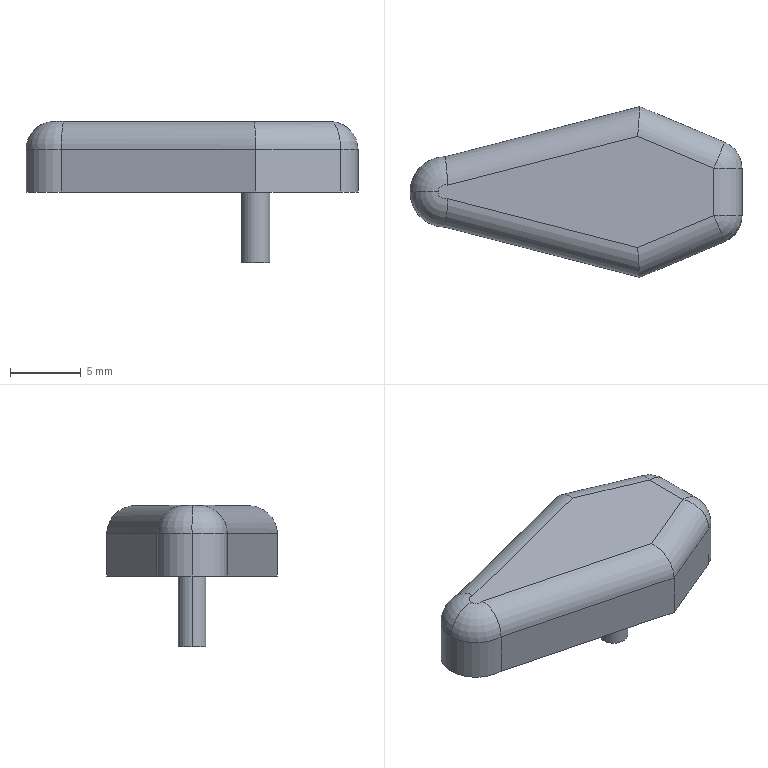Part | SolidWorks | features Fillet 3, Extrusion 1, ICE 1 | 1 solid | 23 faces | box 23.543 x 12.102 x 10 mm | volume 933.083 mm3 | cylinder 11 | plane 8 | torus 2 | sphere 2 | commonest cylinder face diameters 4 x7 2 x2 5 x2
STEP:
#1=CARTESIAN_POINT('',(-2.5,0.,3.));
#2=VERTEX_POINT('',#1);
#3=CARTESIAN_POINT('',(0.,2.5,3.));
#4=VERTEX_POINT('',#3);
#5=CARTESIAN_POINT('',(0.,0.,3.));
#6=DIRECTION('',(0.,0.,-1.));
#7=DIRECTION('',(1.,0.,0.));
#8=AXIS2_PLACEMENT_3D('',#5,#6,#7);
#9=CIRCLE('',#8,2.5);
#10=EDGE_CURVE('',#2,#4,#9,.T.);
#11=ORIENTED_EDGE('',*,*,#10,.F.);
#12=CARTESIAN_POINT('',(-0.5,0.,5.));
#13=VERTEX_POINT('',#12);
#14=CARTESIAN_POINT('',(-0.5,0.,3.));
#15=DIRECTION('',(0.,1.,0.));
#16=DIRECTION('',(-1.,0.,0.));
#17=AXIS2_PLACEMENT_3D('',#14,#15,#16);
#18=CIRCLE('',#17,2.);
#19=EDGE_CURVE('',#2,#13,#18,.T.);
#20=ORIENTED_EDGE('',*,*,#19,.T.);
#21=CARTESIAN_POINT('',(0.1561,0.475,5.));
#22=VERTEX_POINT('',#21);
#23=CARTESIAN_POINT('',(0.,0.,5.));
#24=DIRECTION('',(0.,0.,1.));
#25=DIRECTION('',(1.,0.,0.));
#26=AXIS2_PLACEMENT_3D('',#23,#24,#25);
#27=CIRCLE('',#26,0.5);
#28=EDGE_CURVE('',#22,#13,#27,.T.);
#29=ORIENTED_EDGE('',*,*,#28,.F.);
#30=CARTESIAN_POINT('',(0.,2.5,3.));
#31=CARTESIAN_POINT('',(0.,2.5,3.133));
#32=CARTESIAN_POINT('',(0.001676,2.487,3.264));
#33=CARTESIAN_POINT('',(0.008164,2.435,3.522));
#34=CARTESIAN_POINT('',(0.01306,2.396,3.65));
#35=CARTESIAN_POINT('',(0.02554,2.294,3.893));
#36=CARTESIAN_POINT('',(0.03307,2.232,4.009));
#37=CARTESIAN_POINT('',(0.05029,2.084,4.227));
#38=CARTESIAN_POINT('',(0.06004,1.999,4.33));
#39=CARTESIAN_POINT('',(0.0903,1.718,4.606));
#40=CARTESIAN_POINT('',(0.1129,1.493,4.753));
#41=CARTESIAN_POINT('',(0.1489,1.006,4.949));
#42=CARTESIAN_POINT('',(0.1643,0.7376,5.));
#43=CARTESIAN_POINT('',(0.1561,0.475,5.));
#44=B_SPLINE_CURVE_WITH_KNOTS('',3,(#30,#31,#32,#33,#34,#35,#36,#37,#38,#39,#40,#41,#42,#43),.UNSPECIFIED.,.F.,.F.,(4,2,2,2,2,2,4),(0.,0.0003941,0.0007882,0.001182,0.001576,0.002364,0.003153),.UNSPECIFIED.);
#45=EDGE_CURVE('',#4,#22,#44,.T.);
#46=ORIENTED_EDGE('',*,*,#45,.F.);
#47=EDGE_LOOP('',(#11,#20,#29,#46));
#48=FACE_OUTER_BOUND('',#47,.T.);
#49=CARTESIAN_POINT('',(0.,0.,3.));
#50=DIRECTION('',(0.,0.,1.));
#51=DIRECTION('',(1.,0.,0.));
#52=AXIS2_PLACEMENT_3D('',#49,#50,#51);
#53=TOROIDAL_SURFACE('',#52,0.5,2.);
#54=ADVANCED_FACE('',(#48),#53,.T.);
#55=CARTESIAN_POINT('',(12.798,0.,-5.));
#56=VERTEX_POINT('',#55);
#57=CARTESIAN_POINT('',(14.798,0.,-5.));
#58=VERTEX_POINT('',#57);
#59=CARTESIAN_POINT('',(13.798,0.,-5.));
#60=DIRECTION('',(0.,0.,-1.));
#61=DIRECTION('',(-1.,0.,0.));
#62=AXIS2_PLACEMENT_3D('',#59,#60,#61);
#63=CIRCLE('',#62,1.);
#64=EDGE_CURVE('',#56,#58,#63,.T.);
#65=ORIENTED_EDGE('',*,*,#64,.F.);
#66=CARTESIAN_POINT('',(12.798,0.,0.));
#67=VERTEX_POINT('',#66);
#68=CARTESIAN_POINT('',(12.798,0.,-5.));
#69=DIRECTION('',(0.,0.,1.));
#70=VECTOR('',#69,1000.);
#71=LINE('',#68,#70);
#72=EDGE_CURVE('',#56,#67,#71,.T.);
#73=ORIENTED_EDGE('',*,*,#72,.T.);
#74=CARTESIAN_POINT('',(14.798,0.,0.));
#75=VERTEX_POINT('',#74);
#76=CARTESIAN_POINT('',(13.798,0.,0.));
#77=DIRECTION('',(0.,0.,-1.));
#78=DIRECTION('',(1.,0.,0.));
#79=AXIS2_PLACEMENT_3D('',#76,#77,#78);
#80=CIRCLE('',#79,1.);
#81=EDGE_CURVE('',#67,#75,#80,.T.);
#82=ORIENTED_EDGE('',*,*,#81,.T.);
#83=CARTESIAN_POINT('',(14.798,0.,-5.));
#84=DIRECTION('',(0.,0.,1.));
#85=VECTOR('',#84,1000.);
#86=LINE('',#83,#85);
#87=EDGE_CURVE('',#58,#75,#86,.T.);
#88=ORIENTED_EDGE('',*,*,#87,.F.);
#89=EDGE_LOOP('',(#65,#73,#82,#88));
#90=FACE_OUTER_BOUND('',#89,.T.);
#91=CARTESIAN_POINT('',(13.798,0.,-5.));
#92=DIRECTION('',(0.,0.,1.));
#93=DIRECTION('',(1.,0.,0.));
#94=AXIS2_PLACEMENT_3D('',#91,#92,#93);
#95=CYLINDRICAL_SURFACE('',#94,1.);
#96=ADVANCED_FACE('',(#90),#95,.T.);
#97=CARTESIAN_POINT('',(0.,-2.5,3.));
#98=VERTEX_POINT('',#97);
#99=CARTESIAN_POINT('',(0.,0.,3.));
#100=DIRECTION('',(0.,0.,-1.));
#101=DIRECTION('',(1.,0.,0.));
#102=AXIS2_PLACEMENT_3D('',#99,#100,#101);
#103=CIRCLE('',#102,2.5);
#104=EDGE_CURVE('',#98,#2,#103,.T.);
#105=ORIENTED_EDGE('',*,*,#104,.T.);
#106=CARTESIAN_POINT('',(-2.5,0.,0.));
#107=VERTEX_POINT('',#106);
#108=CARTESIAN_POINT('',(-2.5,0.,5.));
#109=DIRECTION('',(0.,0.,-1.));
#110=VECTOR('',#109,1000.);
#111=LINE('',#108,#110);
#112=EDGE_CURVE('',#2,#107,#111,.T.);
#113=ORIENTED_EDGE('',*,*,#112,.T.);
#114=CARTESIAN_POINT('',(0.,-2.5,0.));
#115=VERTEX_POINT('',#114);
#116=CARTESIAN_POINT('',(0.,0.,0.));
#117=DIRECTION('',(0.,0.,1.));
#118=DIRECTION('',(1.,0.,0.));
#119=AXIS2_PLACEMENT_3D('',#116,#117,#118);
#120=CIRCLE('',#119,2.5);
#121=EDGE_CURVE('',#107,#115,#120,.T.);
#122=ORIENTED_EDGE('',*,*,#121,.T.);
#123=CARTESIAN_POINT('',(0.,-2.5,5.));
#124=DIRECTION('',(0.,0.,-1.));
#125=VECTOR('',#124,1000.);
#126=LINE('',#123,#125);
#127=EDGE_CURVE('',#98,#115,#126,.T.);
#128=ORIENTED_EDGE('',*,*,#127,.F.);
#129=EDGE_LOOP('',(#105,#113,#122,#128));
#130=FACE_OUTER_BOUND('',#129,.T.);
#131=CARTESIAN_POINT('',(0.,0.,5.));
#132=DIRECTION('',(0.,0.,-1.));
#133=DIRECTION('',(-1.,0.,0.));
#134=AXIS2_PLACEMENT_3D('',#131,#132,#133);
#135=CYLINDRICAL_SURFACE('',#134,2.5);
#136=ADVANCED_FACE('',(#130),#135,.T.);
#137=ORIENTED_EDGE('',*,*,#112,.F.);
#138=ORIENTED_EDGE('',*,*,#10,.T.);
#139=CARTESIAN_POINT('',(0.,2.5,0.));
#140=VERTEX_POINT('',#139);
#141=CARTESIAN_POINT('',(0.,2.5,5.));
#142=DIRECTION('',(0.,0.,-1.));
#143=VECTOR('',#142,1000.);
#144=LINE('',#141,#143);
#145=EDGE_CURVE('',#4,#140,#144,.T.);
#146=ORIENTED_EDGE('',*,*,#145,.T.);
#147=CARTESIAN_POINT('',(0.,0.,0.));
#148=DIRECTION('',(0.,0.,1.));
#149=DIRECTION('',(1.,0.,0.));
#150=AXIS2_PLACEMENT_3D('',#147,#148,#149);
#151=CIRCLE('',#150,2.5);
#152=EDGE_CURVE('',#140,#107,#151,.T.);
#153=ORIENTED_EDGE('',*,*,#152,.T.);
#154=EDGE_LOOP('',(#137,#138,#146,#153));
#155=FACE_OUTER_BOUND('',#154,.T.);
#156=CARTESIAN_POINT('',(0.,0.,5.));
#157=DIRECTION('',(0.,0.,-1.));
#158=DIRECTION('',(-1.,0.,0.));
#159=AXIS2_PLACEMENT_3D('',#156,#157,#158);
#160=CYLINDRICAL_SURFACE('',#159,2.5);
#161=ADVANCED_FACE('',(#155),#160,.T.);
#162=CARTESIAN_POINT('',(13.798,-6.051,3.));
#163=VERTEX_POINT('',#162);
#164=CARTESIAN_POINT('',(13.798,-6.051,0.));
#165=VERTEX_POINT('',#164);
#166=CARTESIAN_POINT('',(13.798,-6.051,5.));
#167=DIRECTION('',(0.,0.,-1.));
#168=VECTOR('',#167,1000.);
#169=LINE('',#166,#168);
#170=EDGE_CURVE('',#163,#165,#169,.T.);
#171=ORIENTED_EDGE('',*,*,#170,.F.);
#172=CARTESIAN_POINT('',(0.,-2.5,3.));
#173=DIRECTION('',(-0.9684,0.2492,0.));
#174=VECTOR('',#173,1000.);
#175=LINE('',#172,#174);
#176=EDGE_CURVE('',#163,#98,#175,.T.);
#177=ORIENTED_EDGE('',*,*,#176,.T.);
#178=ORIENTED_EDGE('',*,*,#127,.T.);
#179=CARTESIAN_POINT('',(0.,-2.5,0.));
#180=DIRECTION('',(0.9684,-0.2492,0.));
#181=VECTOR('',#180,1000.);
#182=LINE('',#179,#181);
#183=EDGE_CURVE('',#115,#165,#182,.T.);
#184=ORIENTED_EDGE('',*,*,#183,.T.);
#185=EDGE_LOOP('',(#171,#177,#178,#184));
#186=FACE_OUTER_BOUND('',#185,.T.);
#187=CARTESIAN_POINT('',(0.,-2.5,5.));
#188=DIRECTION('',(0.2492,0.9684,0.));
#189=DIRECTION('',(-0.9684,0.2492,0.));
#190=AXIS2_PLACEMENT_3D('',#187,#188,#189);
#191=PLANE('',#190);
#192=ADVANCED_FACE('',(#186),#191,.F.);
#193=CARTESIAN_POINT('',(19.816,-3.528,0.));
#194=VERTEX_POINT('',#193);
#195=CARTESIAN_POINT('',(13.798,-6.051,0.));
#196=DIRECTION('',(0.9223,0.3866,0.));
#197=VECTOR('',#196,1000.);
#198=LINE('',#195,#197);
#199=EDGE_CURVE('',#165,#194,#198,.T.);
#200=ORIENTED_EDGE('',*,*,#199,.T.);
#201=CARTESIAN_POINT('',(19.816,-3.528,3.));
#202=VERTEX_POINT('',#201);
#203=CARTESIAN_POINT('',(19.816,-3.528,5.));
#204=DIRECTION('',(0.,0.,1.));
#205=VECTOR('',#204,1000.);
#206=LINE('',#203,#205);
#207=EDGE_CURVE('',#194,#202,#206,.T.);
#208=ORIENTED_EDGE('',*,*,#207,.T.);
#209=CARTESIAN_POINT('',(13.798,-6.051,3.));
#210=DIRECTION('',(-0.9223,-0.3866,0.));
#211=VECTOR('',#210,1000.);
#212=LINE('',#209,#211);
#213=EDGE_CURVE('',#202,#163,#212,.T.);
#214=ORIENTED_EDGE('',*,*,#213,.T.);
#215=ORIENTED_EDGE('',*,*,#170,.T.);
#216=EDGE_LOOP('',(#200,#208,#214,#215));
#217=FACE_OUTER_BOUND('',#216,.T.);
#218=CARTESIAN_POINT('',(13.798,-6.051,5.));
#219=DIRECTION('',(-0.3866,0.9223,0.));
#220=DIRECTION('',(-0.9223,-0.3866,0.));
#221=AXIS2_PLACEMENT_3D('',#218,#219,#220);
#222=PLANE('',#221);
#223=ADVANCED_FACE('',(#217),#222,.F.);
#224=CARTESIAN_POINT('',(21.043,-1.684,0.));
#225=VERTEX_POINT('',#224);
#226=CARTESIAN_POINT('',(21.043,1.684,0.));
#227=VERTEX_POINT('',#226);
#228=CARTESIAN_POINT('',(21.043,3.014,0.));
#229=DIRECTION('',(0.,1.,0.));
#230=VECTOR('',#229,1000.);
#231=LINE('',#228,#230);
#232=EDGE_CURVE('',#225,#227,#231,.T.);
#233=ORIENTED_EDGE('',*,*,#232,.T.);
#234=CARTESIAN_POINT('',(21.043,1.684,3.));
#235=VERTEX_POINT('',#234);
#236=CARTESIAN_POINT('',(21.043,1.684,5.));
#237=DIRECTION('',(0.,0.,1.));
#238=VECTOR('',#237,1000.);
#239=LINE('',#236,#238);
#240=EDGE_CURVE('',#227,#235,#239,.T.);
#241=ORIENTED_EDGE('',*,*,#240,.T.);
#242=CARTESIAN_POINT('',(21.043,-1.684,3.));
#243=VERTEX_POINT('',#242);
#244=CARTESIAN_POINT('',(21.043,-3.014,3.));
#245=DIRECTION('',(0.,-1.,0.));
#246=VECTOR('',#245,1000.);
#247=LINE('',#244,#246);
#248=EDGE_CURVE('',#235,#243,#247,.T.);
#249=ORIENTED_EDGE('',*,*,#248,.T.);
#250=CARTESIAN_POINT('',(21.043,-1.684,5.));
#251=DIRECTION('',(0.,0.,-1.));
#252=VECTOR('',#251,1000.);
#253=LINE('',#250,#252);
#254=EDGE_CURVE('',#243,#225,#253,.T.);
#255=ORIENTED_EDGE('',*,*,#254,.T.);
#256=EDGE_LOOP('',(#233,#241,#249,#255));
#257=FACE_OUTER_BOUND('',#256,.T.);
#258=CARTESIAN_POINT('',(21.043,3.014,5.));
#259=DIRECTION('',(-1.,0.,0.));
#260=DIRECTION('',(0.,0.,1.));
#261=AXIS2_PLACEMENT_3D('',#258,#259,#260);
#262=PLANE('',#261);
#263=ADVANCED_FACE('',(#257),#262,.F.);
#264=CARTESIAN_POINT('',(13.798,6.051,3.));
#265=VERTEX_POINT('',#264);
#266=CARTESIAN_POINT('',(19.816,3.528,3.));
#267=VERTEX_POINT('',#266);
#268=CARTESIAN_POINT('',(19.043,3.852,3.));
#269=DIRECTION('',(0.9223,-0.3866,0.));
#270=VECTOR('',#269,1000.);
#271=LINE('',#268,#270);
#272=EDGE_CURVE('',#265,#267,#271,.T.);
#273=ORIENTED_EDGE('',*,*,#272,.T.);
#274=CARTESIAN_POINT('',(19.816,3.528,0.));
#275=VERTEX_POINT('',#274);
#276=CARTESIAN_POINT('',(19.816,3.528,5.));
#277=DIRECTION('',(0.,0.,-1.));
#278=VECTOR('',#277,1000.);
#279=LINE('',#276,#278);
#280=EDGE_CURVE('',#267,#275,#279,.T.);
#281=ORIENTED_EDGE('',*,*,#280,.T.);
#282=CARTESIAN_POINT('',(13.798,6.051,0.));
#283=VERTEX_POINT('',#282);
#284=CARTESIAN_POINT('',(13.798,6.051,0.));
#285=DIRECTION('',(-0.9223,0.3866,0.));
#286=VECTOR('',#285,1000.);
#287=LINE('',#284,#286);
#288=EDGE_CURVE('',#275,#283,#287,.T.);
#289=ORIENTED_EDGE('',*,*,#288,.T.);
#290=CARTESIAN_POINT('',(13.798,6.051,5.));
#291=DIRECTION('',(0.,0.,-1.));
#292=VECTOR('',#291,1000.);
#293=LINE('',#290,#292);
#294=EDGE_CURVE('',#265,#283,#293,.T.);
#295=ORIENTED_EDGE('',*,*,#294,.F.);
#296=EDGE_LOOP('',(#273,#281,#289,#295));
#297=FACE_OUTER_BOUND('',#296,.T.);
#298=CARTESIAN_POINT('',(13.798,6.051,5.));
#299=DIRECTION('',(-0.3866,-0.9223,0.));
#300=DIRECTION('',(0.9223,-0.3866,0.));
#301=AXIS2_PLACEMENT_3D('',#298,#299,#300);
#302=PLANE('',#301);
#303=ADVANCED_FACE('',(#297),#302,.F.);
#304=ORIENTED_EDGE('',*,*,#145,.F.);
#305=CARTESIAN_POINT('',(13.798,6.051,3.));
#306=DIRECTION('',(0.9684,0.2492,0.));
#307=VECTOR('',#306,1000.);
#308=LINE('',#305,#307);
#309=EDGE_CURVE('',#4,#265,#308,.T.);
#310=ORIENTED_EDGE('',*,*,#309,.T.);
#311=ORIENTED_EDGE('',*,*,#294,.T.);
#312=CARTESIAN_POINT('',(0.,2.5,0.));
#313=DIRECTION('',(-0.9684,-0.2492,0.));
#314=VECTOR('',#313,1000.);
#315=LINE('',#312,#314);
#316=EDGE_CURVE('',#283,#140,#315,.T.);
#317=ORIENTED_EDGE('',*,*,#316,.T.);
#318=EDGE_LOOP('',(#304,#310,#311,#317));
#319=FACE_OUTER_BOUND('',#318,.T.);
#320=CARTESIAN_POINT('',(0.,2.5,5.));
#321=DIRECTION('',(0.2492,-0.9684,0.));
#322=DIRECTION('',(0.9684,0.2492,0.));
#323=AXIS2_PLACEMENT_3D('',#320,#321,#322);
#324=PLANE('',#323);
#325=ADVANCED_FACE('',(#319),#324,.F.);
#326=ORIENTED_EDGE('',*,*,#28,.T.);
#327=CARTESIAN_POINT('',(0.1561,-0.475,5.));
#328=VERTEX_POINT('',#327);
#329=CARTESIAN_POINT('',(0.,0.,5.));
#330=DIRECTION('',(0.,0.,1.));
#331=DIRECTION('',(1.,0.,0.));
#332=AXIS2_PLACEMENT_3D('',#329,#330,#331);
#333=CIRCLE('',#332,0.5);
#334=EDGE_CURVE('',#13,#328,#333,.T.);
#335=ORIENTED_EDGE('',*,*,#334,.T.);
#336=CARTESIAN_POINT('',(13.645,-3.946,5.));
#337=VERTEX_POINT('',#336);
#338=CARTESIAN_POINT('',(14.296,-4.114,5.));
#339=DIRECTION('',(0.9684,-0.2492,0.));
#340=VECTOR('',#339,1000.);
#341=LINE('',#338,#340);
#342=EDGE_CURVE('',#328,#337,#341,.T.);
#343=ORIENTED_EDGE('',*,*,#342,.T.);
#344=CARTESIAN_POINT('',(19.043,-1.684,5.));
#345=VERTEX_POINT('',#344);
#346=CARTESIAN_POINT('',(18.27,-2.008,5.));
#347=DIRECTION('',(0.9223,0.3866,0.));
#348=VECTOR('',#347,1000.);
#349=LINE('',#346,#348);
#350=EDGE_CURVE('',#337,#345,#349,.T.);
#351=ORIENTED_EDGE('',*,*,#350,.T.);
#352=CARTESIAN_POINT('',(19.043,1.684,5.));
#353=VERTEX_POINT('',#352);
#354=CARTESIAN_POINT('',(19.043,3.014,5.));
#355=DIRECTION('',(0.,1.,0.));
#356=VECTOR('',#355,1000.);
#357=LINE('',#354,#356);
#358=EDGE_CURVE('',#345,#353,#357,.T.);
#359=ORIENTED_EDGE('',*,*,#358,.T.);
#360=CARTESIAN_POINT('',(13.645,3.946,5.));
#361=VERTEX_POINT('',#360);
#362=CARTESIAN_POINT('',(13.025,4.206,5.));
#363=DIRECTION('',(-0.9223,0.3866,0.));
#364=VECTOR('',#363,1000.);
#365=LINE('',#362,#364);
#366=EDGE_CURVE('',#353,#361,#365,.T.);
#367=ORIENTED_EDGE('',*,*,#366,.T.);
#368=CARTESIAN_POINT('',(0.4985,0.5631,5.));
#369=DIRECTION('',(-0.9684,-0.2492,0.));
#370=VECTOR('',#369,1000.);
#371=LINE('',#368,#370);
#372=EDGE_CURVE('',#361,#22,#371,.T.);
#373=ORIENTED_EDGE('',*,*,#372,.T.);
#374=EDGE_LOOP('',(#326,#335,#343,#351,#359,#367,#373));
#375=FACE_OUTER_BOUND('',#374,.T.);
#376=CARTESIAN_POINT('',(0.,0.,5.));
#377=DIRECTION('',(0.,0.,1.));
#378=DIRECTION('',(1.,0.,0.));
#379=AXIS2_PLACEMENT_3D('',#376,#377,#378);
#380=PLANE('',#379);
#381=ADVANCED_FACE('',(#375),#380,.T.);
#382=CARTESIAN_POINT('',(13.798,0.,0.));
#383=DIRECTION('',(0.,0.,-1.));
#384=DIRECTION('',(1.,0.,0.));
#385=AXIS2_PLACEMENT_3D('',#382,#383,#384);
#386=CIRCLE('',#385,1.);
#387=EDGE_CURVE('',#75,#67,#386,.T.);
#388=ORIENTED_EDGE('',*,*,#387,.F.);
#389=ORIENTED_EDGE('',*,*,#81,.F.);
#390=EDGE_LOOP('',(#388,#389));
#391=FACE_BOUND('',#390,.T.);
#392=ORIENTED_EDGE('',*,*,#288,.F.);
#393=CARTESIAN_POINT('',(19.043,1.684,0.));
#394=DIRECTION('',(0.,0.,-1.));
#395=DIRECTION('',(1.,0.,0.));
#396=AXIS2_PLACEMENT_3D('',#393,#394,#395);
#397=CIRCLE('',#396,2.);
#398=EDGE_CURVE('',#275,#227,#397,.T.);
#399=ORIENTED_EDGE('',*,*,#398,.T.);
#400=ORIENTED_EDGE('',*,*,#232,.F.);
#401=CARTESIAN_POINT('',(19.043,-1.684,0.));
#402=DIRECTION('',(0.,0.,-1.));
#403=DIRECTION('',(1.,0.,0.));
#404=AXIS2_PLACEMENT_3D('',#401,#402,#403);
#405=CIRCLE('',#404,2.);
#406=EDGE_CURVE('',#225,#194,#405,.T.);
#407=ORIENTED_EDGE('',*,*,#406,.T.);
#408=ORIENTED_EDGE('',*,*,#199,.F.);
#409=ORIENTED_EDGE('',*,*,#183,.F.);
#410=ORIENTED_EDGE('',*,*,#121,.F.);
#411=ORIENTED_EDGE('',*,*,#152,.F.);
#412=ORIENTED_EDGE('',*,*,#316,.F.);
#413=EDGE_LOOP('',(#392,#399,#400,#407,#408,#409,#410,#411,#412));
#414=FACE_OUTER_BOUND('',#413,.T.);
#415=CARTESIAN_POINT('',(0.,0.,0.));
#416=DIRECTION('',(0.,0.,1.));
#417=DIRECTION('',(1.,0.,0.));
#418=AXIS2_PLACEMENT_3D('',#415,#416,#417);
#419=PLANE('',#418);
#420=ADVANCED_FACE('',(#391,#414),#419,.F.);
#421=ORIENTED_EDGE('',*,*,#72,.F.);
#422=CARTESIAN_POINT('',(13.798,0.,-5.));
#423=DIRECTION('',(0.,0.,-1.));
#424=DIRECTION('',(-1.,0.,0.));
#425=AXIS2_PLACEMENT_3D('',#422,#423,#424);
#426=CIRCLE('',#425,1.);
#427=EDGE_CURVE('',#58,#56,#426,.T.);
#428=ORIENTED_EDGE('',*,*,#427,.F.);
#429=ORIENTED_EDGE('',*,*,#87,.T.);
#430=ORIENTED_EDGE('',*,*,#387,.T.);
#431=EDGE_LOOP('',(#421,#428,#429,#430));
#432=FACE_OUTER_BOUND('',#431,.T.);
#433=CARTESIAN_POINT('',(13.798,0.,-5.));
#434=DIRECTION('',(0.,0.,1.));
#435=DIRECTION('',(1.,0.,0.));
#436=AXIS2_PLACEMENT_3D('',#433,#434,#435);
#437=CYLINDRICAL_SURFACE('',#436,1.);
#438=ADVANCED_FACE('',(#432),#437,.T.);
#439=ORIENTED_EDGE('',*,*,#427,.T.);
#440=ORIENTED_EDGE('',*,*,#64,.T.);
#441=EDGE_LOOP('',(#439,#440));
#442=FACE_OUTER_BOUND('',#441,.T.);
#443=CARTESIAN_POINT('',(13.798,0.,-5.));
#444=DIRECTION('',(0.,0.,-1.));
#445=DIRECTION('',(-1.,0.,0.));
#446=AXIS2_PLACEMENT_3D('',#443,#444,#445);
#447=PLANE('',#446);
#448=ADVANCED_FACE('',(#442),#447,.T.);
#449=ORIENTED_EDGE('',*,*,#248,.F.);
#450=CARTESIAN_POINT('',(19.043,1.684,3.));
#451=DIRECTION('',(0.,-1.,0.));
#452=DIRECTION('',(0.,0.,-1.));
#453=AXIS2_PLACEMENT_3D('',#450,#451,#452);
#454=CIRCLE('',#453,2.);
#455=EDGE_CURVE('',#235,#353,#454,.T.);
#456=ORIENTED_EDGE('',*,*,#455,.T.);
#457=ORIENTED_EDGE('',*,*,#358,.F.);
#458=CARTESIAN_POINT('',(19.043,-1.684,3.));
#459=DIRECTION('',(0.,1.,0.));
#460=DIRECTION('',(0.,0.,-1.));
#461=AXIS2_PLACEMENT_3D('',#458,#459,#460);
#462=CIRCLE('',#461,2.);
#463=EDGE_CURVE('',#345,#243,#462,.T.);
#464=ORIENTED_EDGE('',*,*,#463,.T.);
#465=EDGE_LOOP('',(#449,#456,#457,#464));
#466=FACE_OUTER_BOUND('',#465,.T.);
#467=CARTESIAN_POINT('',(19.043,0.,3.));
#468=DIRECTION('',(0.,-1.,0.));
#469=DIRECTION('',(0.,0.,-1.));
#470=AXIS2_PLACEMENT_3D('',#467,#468,#469);
#471=CYLINDRICAL_SURFACE('',#470,2.);
#472=ADVANCED_FACE('',(#466),#471,.T.);
#473=ORIENTED_EDGE('',*,*,#342,.F.);
#474=CARTESIAN_POINT('',(0.1561,-0.475,5.));
#475=CARTESIAN_POINT('',(0.1643,-0.7395,5.));
#476=CARTESIAN_POINT('',(0.1489,-1.006,4.949));
#477=CARTESIAN_POINT('',(0.1129,-1.493,4.753));
#478=CARTESIAN_POINT('',(0.09029,-1.718,4.606));
#479=CARTESIAN_POINT('',(0.06003,-1.999,4.33));
#480=CARTESIAN_POINT('',(0.05029,-2.084,4.227));
#481=CARTESIAN_POINT('',(0.03307,-2.232,4.009));
#482=CARTESIAN_POINT('',(0.02554,-2.294,3.893));
#483=CARTESIAN_POINT('',(0.01306,-2.396,3.65));
#484=CARTESIAN_POINT('',(0.008163,-2.435,3.522));
#485=CARTESIAN_POINT('',(0.001676,-2.487,3.264));
#486=CARTESIAN_POINT('',(0.,-2.5,3.133));
#487=CARTESIAN_POINT('',(0.,-2.5,3.));
#488=B_SPLINE_CURVE_WITH_KNOTS('',3,(#474,#475,#476,#477,#478,#479,#480,#481,#482,#483,#484,#485,#486,#487),.UNSPECIFIED.,.F.,.F.,(4,2,2,2,2,2,4),(-0.00001218,0.0007817,0.001576,0.001973,0.002369,0.002766,0.003163),.UNSPECIFIED.);
#489=EDGE_CURVE('',#328,#98,#488,.T.);
#490=ORIENTED_EDGE('',*,*,#489,.T.);
#491=ORIENTED_EDGE('',*,*,#176,.F.);
#492=CARTESIAN_POINT('',(13.645,-3.946,5.));
#493=CARTESIAN_POINT('',(13.734,-5.179,5.));
#494=CARTESIAN_POINT('',(13.798,-6.051,4.172));
#495=CARTESIAN_POINT('',(13.798,-6.051,3.));
#496=(BOUNDED_CURVE()B_SPLINE_CURVE(3,(#492,#493,#494,#495),.UNSPECIFIED.,.F.,.T.)B_SPLINE_CURVE_WITH_KNOTS((4,4),(1.571,3.142),.UNSPECIFIED.)CURVE()GEOMETRIC_REPRESENTATION_ITEM()RATIONAL_B_SPLINE_CURVE((1.,0.8047,0.8047,1.))REPRESENTATION_ITEM(''));
#497=EDGE_CURVE('',#337,#163,#496,.T.);
#498=ORIENTED_EDGE('',*,*,#497,.F.);
#499=EDGE_LOOP('',(#473,#490,#491,#498));
#500=FACE_OUTER_BOUND('',#499,.T.);
#501=CARTESIAN_POINT('',(-0.105,-0.4078,3.));
#502=DIRECTION('',(-0.9684,0.2492,0.));
#503=DIRECTION('',(-0.2492,-0.9684,0.));
#504=AXIS2_PLACEMENT_3D('',#501,#502,#503);
#505=CYLINDRICAL_SURFACE('',#504,2.);
#506=ADVANCED_FACE('',(#500),#505,.T.);
#507=CARTESIAN_POINT('',(19.043,-1.684,3.));
#508=DIRECTION('',(0.9223,0.3866,0.));
#509=DIRECTION('',(-0.3866,0.9223,0.));
#510=AXIS2_PLACEMENT_3D('',#507,#508,#509);
#511=CIRCLE('',#510,2.);
#512=EDGE_CURVE('',#345,#202,#511,.T.);
#513=ORIENTED_EDGE('',*,*,#512,.F.);
#514=ORIENTED_EDGE('',*,*,#350,.F.);
#515=ORIENTED_EDGE('',*,*,#497,.T.);
#516=ORIENTED_EDGE('',*,*,#213,.F.);
#517=EDGE_LOOP('',(#513,#514,#515,#516));
#518=FACE_OUTER_BOUND('',#517,.T.);
#519=CARTESIAN_POINT('',(3.446,-8.221,3.));
#520=DIRECTION('',(-0.9223,-0.3866,0.));
#521=DIRECTION('',(0.3866,-0.9223,0.));
#522=AXIS2_PLACEMENT_3D('',#519,#520,#521);
#523=CYLINDRICAL_SURFACE('',#522,2.);
#524=ADVANCED_FACE('',(#518),#523,.T.);
#525=ORIENTED_EDGE('',*,*,#463,.F.);
#526=ORIENTED_EDGE('',*,*,#512,.T.);
#527=CARTESIAN_POINT('',(19.043,-1.684,3.));
#528=DIRECTION('',(0.,0.,-1.));
#529=DIRECTION('',(-1.,0.,0.));
#530=AXIS2_PLACEMENT_3D('',#527,#528,#529);
#531=CIRCLE('',#530,2.);
#532=EDGE_CURVE('',#243,#202,#531,.T.);
#533=ORIENTED_EDGE('',*,*,#532,.F.);
#534=EDGE_LOOP('',(#525,#526,#533));
#535=FACE_OUTER_BOUND('',#534,.T.);
#536=CARTESIAN_POINT('',(19.043,-1.684,3.));
#537=DIRECTION('',(0.,0.,1.));
#538=DIRECTION('',(-0.9223,-0.3866,0.));
#539=AXIS2_PLACEMENT_3D('',#536,#537,#538);
#540=SPHERICAL_SURFACE('',#539,2.);
#541=ADVANCED_FACE('',(#535),#540,.T.);
#542=ORIENTED_EDGE('',*,*,#532,.T.);
#543=ORIENTED_EDGE('',*,*,#207,.F.);
#544=ORIENTED_EDGE('',*,*,#406,.F.);
#545=ORIENTED_EDGE('',*,*,#254,.F.);
#546=EDGE_LOOP('',(#542,#543,#544,#545));
#547=FACE_OUTER_BOUND('',#546,.T.);
#548=CARTESIAN_POINT('',(19.043,-1.684,5.));
#549=DIRECTION('',(0.,0.,-1.));
#550=DIRECTION('',(-1.,0.,0.));
#551=AXIS2_PLACEMENT_3D('',#548,#549,#550);
#552=CYLINDRICAL_SURFACE('',#551,2.);
#553=ADVANCED_FACE('',(#547),#552,.T.);
#554=ORIENTED_EDGE('',*,*,#19,.F.);
#555=ORIENTED_EDGE('',*,*,#104,.F.);
#556=ORIENTED_EDGE('',*,*,#489,.F.);
#557=ORIENTED_EDGE('',*,*,#334,.F.);
#558=EDGE_LOOP('',(#554,#555,#556,#557));
#559=FACE_OUTER_BOUND('',#558,.T.);
#560=CARTESIAN_POINT('',(0.,0.,3.));
#561=DIRECTION('',(0.,0.,1.));
#562=DIRECTION('',(1.,0.,0.));
#563=AXIS2_PLACEMENT_3D('',#560,#561,#562);
#564=TOROIDAL_SURFACE('',#563,0.5,2.);
#565=ADVANCED_FACE('',(#559),#564,.T.);
#566=ORIENTED_EDGE('',*,*,#45,.T.);
#567=ORIENTED_EDGE('',*,*,#372,.F.);
#568=CARTESIAN_POINT('',(13.798,6.051,3.));
#569=CARTESIAN_POINT('',(13.798,6.051,4.172));
#570=CARTESIAN_POINT('',(13.734,5.179,5.));
#571=CARTESIAN_POINT('',(13.645,3.946,5.));
#572=(BOUNDED_CURVE()B_SPLINE_CURVE(3,(#568,#569,#570,#571),.UNSPECIFIED.,.F.,.T.)B_SPLINE_CURVE_WITH_KNOTS((4,4),(3.142,4.712),.UNSPECIFIED.)CURVE()GEOMETRIC_REPRESENTATION_ITEM()RATIONAL_B_SPLINE_CURVE((1.,0.8047,0.8047,1.))REPRESENTATION_ITEM(''));
#573=EDGE_CURVE('',#265,#361,#572,.T.);
#574=ORIENTED_EDGE('',*,*,#573,.F.);
#575=ORIENTED_EDGE('',*,*,#309,.F.);
#576=EDGE_LOOP('',(#566,#567,#574,#575));
#577=FACE_OUTER_BOUND('',#576,.T.);
#578=CARTESIAN_POINT('',(-0.105,0.4078,3.));
#579=DIRECTION('',(0.9684,0.2492,0.));
#580=DIRECTION('',(-0.2492,0.9684,0.));
#581=AXIS2_PLACEMENT_3D('',#578,#579,#580);
#582=CYLINDRICAL_SURFACE('',#581,2.);
#583=ADVANCED_FACE('',(#577),#582,.T.);
#584=ORIENTED_EDGE('',*,*,#573,.T.);
#585=ORIENTED_EDGE('',*,*,#366,.F.);
#586=CARTESIAN_POINT('',(19.043,1.684,3.));
#587=DIRECTION('',(0.9223,-0.3866,0.));
#588=DIRECTION('',(0.3866,0.9223,0.));
#589=AXIS2_PLACEMENT_3D('',#586,#587,#588);
#590=CIRCLE('',#589,2.);
#591=EDGE_CURVE('',#267,#353,#590,.T.);
#592=ORIENTED_EDGE('',*,*,#591,.F.);
#593=ORIENTED_EDGE('',*,*,#272,.F.);
#594=EDGE_LOOP('',(#584,#585,#592,#593));
#595=FACE_OUTER_BOUND('',#594,.T.);
#596=CARTESIAN_POINT('',(3.446,8.221,3.));
#597=DIRECTION('',(0.9223,-0.3866,0.));
#598=DIRECTION('',(0.3866,0.9223,0.));
#599=AXIS2_PLACEMENT_3D('',#596,#597,#598);
#600=CYLINDRICAL_SURFACE('',#599,2.);
#601=ADVANCED_FACE('',(#595),#600,.T.);
#602=ORIENTED_EDGE('',*,*,#591,.T.);
#603=ORIENTED_EDGE('',*,*,#455,.F.);
#604=CARTESIAN_POINT('',(19.043,1.684,3.));
#605=DIRECTION('',(0.,0.,-1.));
#606=DIRECTION('',(-1.,0.,0.));
#607=AXIS2_PLACEMENT_3D('',#604,#605,#606);
#608=CIRCLE('',#607,2.);
#609=EDGE_CURVE('',#267,#235,#608,.T.);
#610=ORIENTED_EDGE('',*,*,#609,.F.);
#611=EDGE_LOOP('',(#602,#603,#610));
#612=FACE_OUTER_BOUND('',#611,.T.);
#613=CARTESIAN_POINT('',(19.043,1.684,3.));
#614=DIRECTION('',(0.,0.,1.));
#615=DIRECTION('',(0.9223,-0.3866,0.));
#616=AXIS2_PLACEMENT_3D('',#613,#614,#615);
#617=SPHERICAL_SURFACE('',#616,2.);
#618=ADVANCED_FACE('',(#612),#617,.T.);
#619=ORIENTED_EDGE('',*,*,#609,.T.);
#620=ORIENTED_EDGE('',*,*,#240,.F.);
#621=ORIENTED_EDGE('',*,*,#398,.F.);
#622=ORIENTED_EDGE('',*,*,#280,.F.);
#623=EDGE_LOOP('',(#619,#620,#621,#622));
#624=FACE_OUTER_BOUND('',#623,.T.);
#625=CARTESIAN_POINT('',(19.043,1.684,5.));
#626=DIRECTION('',(0.,0.,-1.));
#627=DIRECTION('',(-1.,0.,0.));
#628=AXIS2_PLACEMENT_3D('',#625,#626,#627);
#629=CYLINDRICAL_SURFACE('',#628,2.);
#630=ADVANCED_FACE('',(#624),#629,.T.);
#631=CLOSED_SHELL('',(#54,#96,#136,#161,#192,#223,#263,#303,#325,#381,#420,#438,#448,#472,#506,#524,#541,#553,#565,#583,#601,#618,#630));
#632=MANIFOLD_SOLID_BREP('',#631);
#633=CARTESIAN_POINT('',(0.,0.,0.));
#634=DIRECTION('',(0.,0.,1.));
#635=DIRECTION('',(1.,0.,0.));
#636=AXIS2_PLACEMENT_3D('',#633,#634,#635);
#637=(LENGTH_UNIT()NAMED_UNIT(*)SI_UNIT(.MILLI.,.METRE.));
#638=UNCERTAINTY_MEASURE_WITH_UNIT(LENGTH_MEASURE(0.00001),#637,'','');
#639=(NAMED_UNIT(*)PLANE_ANGLE_UNIT()SI_UNIT($,.RADIAN.));
#640=(NAMED_UNIT(*)SI_UNIT($,.STERADIAN.)SOLID_ANGLE_UNIT());
#641=(GEOMETRIC_REPRESENTATION_CONTEXT(3)GLOBAL_UNCERTAINTY_ASSIGNED_CONTEXT((#638))GLOBAL_UNIT_ASSIGNED_CONTEXT((#637,#639,#640))REPRESENTATION_CONTEXT('',''));
#642=ADVANCED_BREP_SHAPE_REPRESENTATION('',(#632,#636),#641);